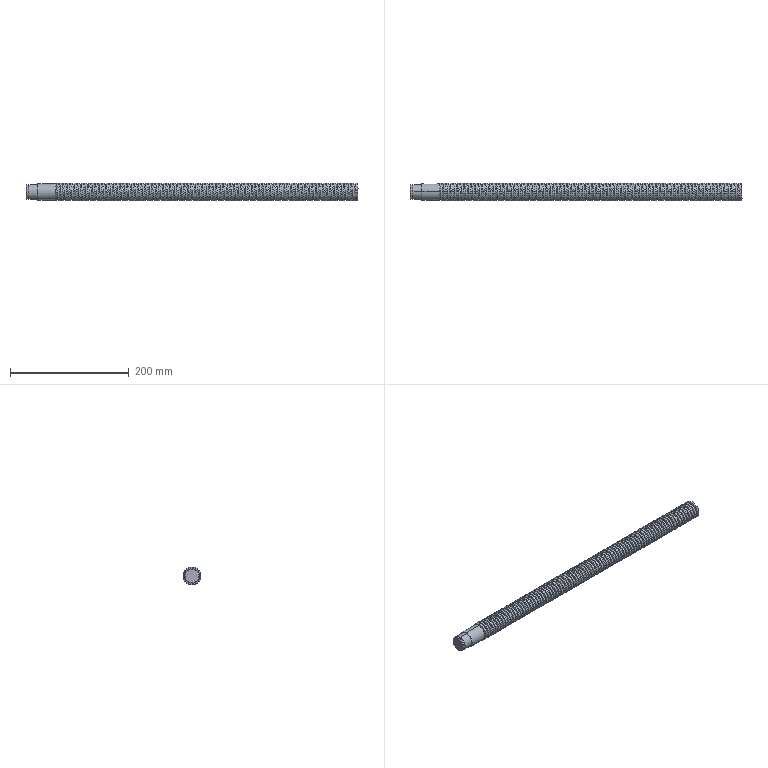Part | SolidWorks | features BaseBody 1 | 1 solid | 197 faces | box 560 x 30 x 30 mm | volume 349970 mm3 | cylinder 182 | plane 10 | spline 3 | cone 2 | commonest cylinder face diameters 30 x172 25 x4 8 x2 23 x2 28 x2